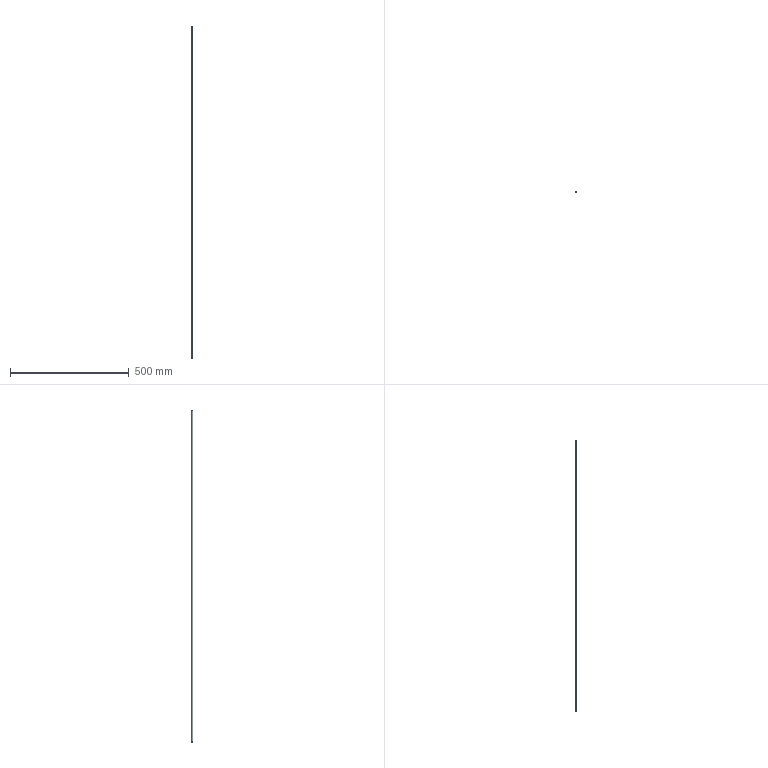Part | SolidWorks | features BaseBody 1 | 1 solid | 4 faces | box 5 x 5 x 1400 mm | volume 27489 mm3 | cylinder 2 | plane 2 | commonest cylinder face diameters 5 x2
STEP:
#1=CARTESIAN_POINT('',(0.,-2.5,1400.));
#2=VERTEX_POINT('',#1);
#3=CARTESIAN_POINT('',(0.,2.5,1400.));
#4=VERTEX_POINT('',#3);
#5=CARTESIAN_POINT('',(0.,0.,1400.));
#6=DIRECTION('',(0.,0.,1.));
#7=DIRECTION('',(0.,1.,0.));
#8=AXIS2_PLACEMENT_3D('',#5,#6,#7);
#9=CIRCLE('',#8,2.5);
#10=EDGE_CURVE('',#2,#4,#9,.T.);
#11=ORIENTED_EDGE('',*,*,#10,.F.);
#12=CARTESIAN_POINT('',(0.,-2.5,0.));
#13=VERTEX_POINT('',#12);
#14=CARTESIAN_POINT('',(0.,-2.5,1400.));
#15=DIRECTION('',(0.,0.,-1.));
#16=VECTOR('',#15,1000.);
#17=LINE('',#14,#16);
#18=EDGE_CURVE('',#2,#13,#17,.T.);
#19=ORIENTED_EDGE('',*,*,#18,.T.);
#20=CARTESIAN_POINT('',(0.,2.5,0.));
#21=VERTEX_POINT('',#20);
#22=CARTESIAN_POINT('',(0.,0.,0.));
#23=DIRECTION('',(0.,0.,-1.));
#24=DIRECTION('',(0.,1.,0.));
#25=AXIS2_PLACEMENT_3D('',#22,#23,#24);
#26=CIRCLE('',#25,2.5);
#27=EDGE_CURVE('',#21,#13,#26,.T.);
#28=ORIENTED_EDGE('',*,*,#27,.F.);
#29=CARTESIAN_POINT('',(0.,2.5,1400.));
#30=DIRECTION('',(0.,0.,-1.));
#31=VECTOR('',#30,1000.);
#32=LINE('',#29,#31);
#33=EDGE_CURVE('',#4,#21,#32,.T.);
#34=ORIENTED_EDGE('',*,*,#33,.F.);
#35=EDGE_LOOP('',(#11,#19,#28,#34));
#36=FACE_OUTER_BOUND('',#35,.T.);
#37=CARTESIAN_POINT('',(0.,0.,1400.));
#38=DIRECTION('',(0.,0.,-1.));
#39=DIRECTION('',(0.,1.,0.));
#40=AXIS2_PLACEMENT_3D('',#37,#38,#39);
#41=CYLINDRICAL_SURFACE('',#40,2.5);
#42=ADVANCED_FACE('',(#36),#41,.T.);
#43=ORIENTED_EDGE('',*,*,#18,.F.);
#44=CARTESIAN_POINT('',(0.,0.,1400.));
#45=DIRECTION('',(0.,0.,1.));
#46=DIRECTION('',(0.,1.,0.));
#47=AXIS2_PLACEMENT_3D('',#44,#45,#46);
#48=CIRCLE('',#47,2.5);
#49=EDGE_CURVE('',#4,#2,#48,.T.);
#50=ORIENTED_EDGE('',*,*,#49,.F.);
#51=ORIENTED_EDGE('',*,*,#33,.T.);
#52=CARTESIAN_POINT('',(0.,0.,0.));
#53=DIRECTION('',(0.,0.,-1.));
#54=DIRECTION('',(0.,1.,0.));
#55=AXIS2_PLACEMENT_3D('',#52,#53,#54);
#56=CIRCLE('',#55,2.5);
#57=EDGE_CURVE('',#13,#21,#56,.T.);
#58=ORIENTED_EDGE('',*,*,#57,.F.);
#59=EDGE_LOOP('',(#43,#50,#51,#58));
#60=FACE_OUTER_BOUND('',#59,.T.);
#61=CARTESIAN_POINT('',(0.,0.,1400.));
#62=DIRECTION('',(0.,0.,-1.));
#63=DIRECTION('',(0.,1.,0.));
#64=AXIS2_PLACEMENT_3D('',#61,#62,#63);
#65=CYLINDRICAL_SURFACE('',#64,2.5);
#66=ADVANCED_FACE('',(#60),#65,.T.);
#67=ORIENTED_EDGE('',*,*,#49,.T.);
#68=ORIENTED_EDGE('',*,*,#10,.T.);
#69=EDGE_LOOP('',(#67,#68));
#70=FACE_OUTER_BOUND('',#69,.T.);
#71=CARTESIAN_POINT('',(-2.53,-2.53,1400.));
#72=DIRECTION('',(0.,0.,1.));
#73=DIRECTION('',(1.,0.,0.));
#74=AXIS2_PLACEMENT_3D('',#71,#72,#73);
#75=PLANE('',#74);
#76=ADVANCED_FACE('',(#70),#75,.T.);
#77=ORIENTED_EDGE('',*,*,#27,.T.);
#78=ORIENTED_EDGE('',*,*,#57,.T.);
#79=EDGE_LOOP('',(#77,#78));
#80=FACE_OUTER_BOUND('',#79,.T.);
#81=CARTESIAN_POINT('',(-2.53,-2.53,0.));
#82=DIRECTION('',(0.,0.,1.));
#83=DIRECTION('',(1.,0.,0.));
#84=AXIS2_PLACEMENT_3D('',#81,#82,#83);
#85=PLANE('',#84);
#86=ADVANCED_FACE('',(#80),#85,.F.);
#87=CLOSED_SHELL('',(#42,#66,#76,#86));
#88=MANIFOLD_SOLID_BREP('',#87);
#89=CARTESIAN_POINT('',(0.,0.,0.));
#90=DIRECTION('',(0.,0.,1.));
#91=DIRECTION('',(1.,0.,0.));
#92=AXIS2_PLACEMENT_3D('',#89,#90,#91);
#93=(LENGTH_UNIT()NAMED_UNIT(*)SI_UNIT(.MILLI.,.METRE.));
#94=UNCERTAINTY_MEASURE_WITH_UNIT(LENGTH_MEASURE(0.00001),#93,'','');
#95=(NAMED_UNIT(*)PLANE_ANGLE_UNIT()SI_UNIT($,.RADIAN.));
#96=(NAMED_UNIT(*)SI_UNIT($,.STERADIAN.)SOLID_ANGLE_UNIT());
#97=(GEOMETRIC_REPRESENTATION_CONTEXT(3)GLOBAL_UNCERTAINTY_ASSIGNED_CONTEXT((#94))GLOBAL_UNIT_ASSIGNED_CONTEXT((#93,#95,#96))REPRESENTATION_CONTEXT('',''));
#98=ADVANCED_BREP_SHAPE_REPRESENTATION('',(#88,#92),#97);